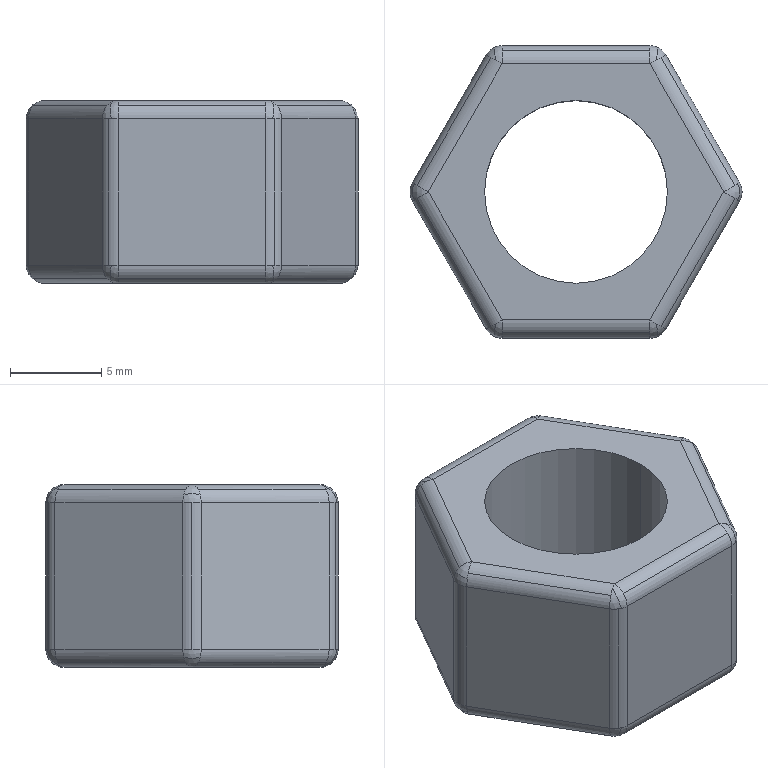Part | SolidWorks | features BaseBody 1 | 1 solid | 70 faces | box 18.166 x 16 x 10 mm | volume 1405 mm3 | cylinder 38 | sphere 24 | plane 8 | commonest cylinder face diameters 2 x36 10 x2